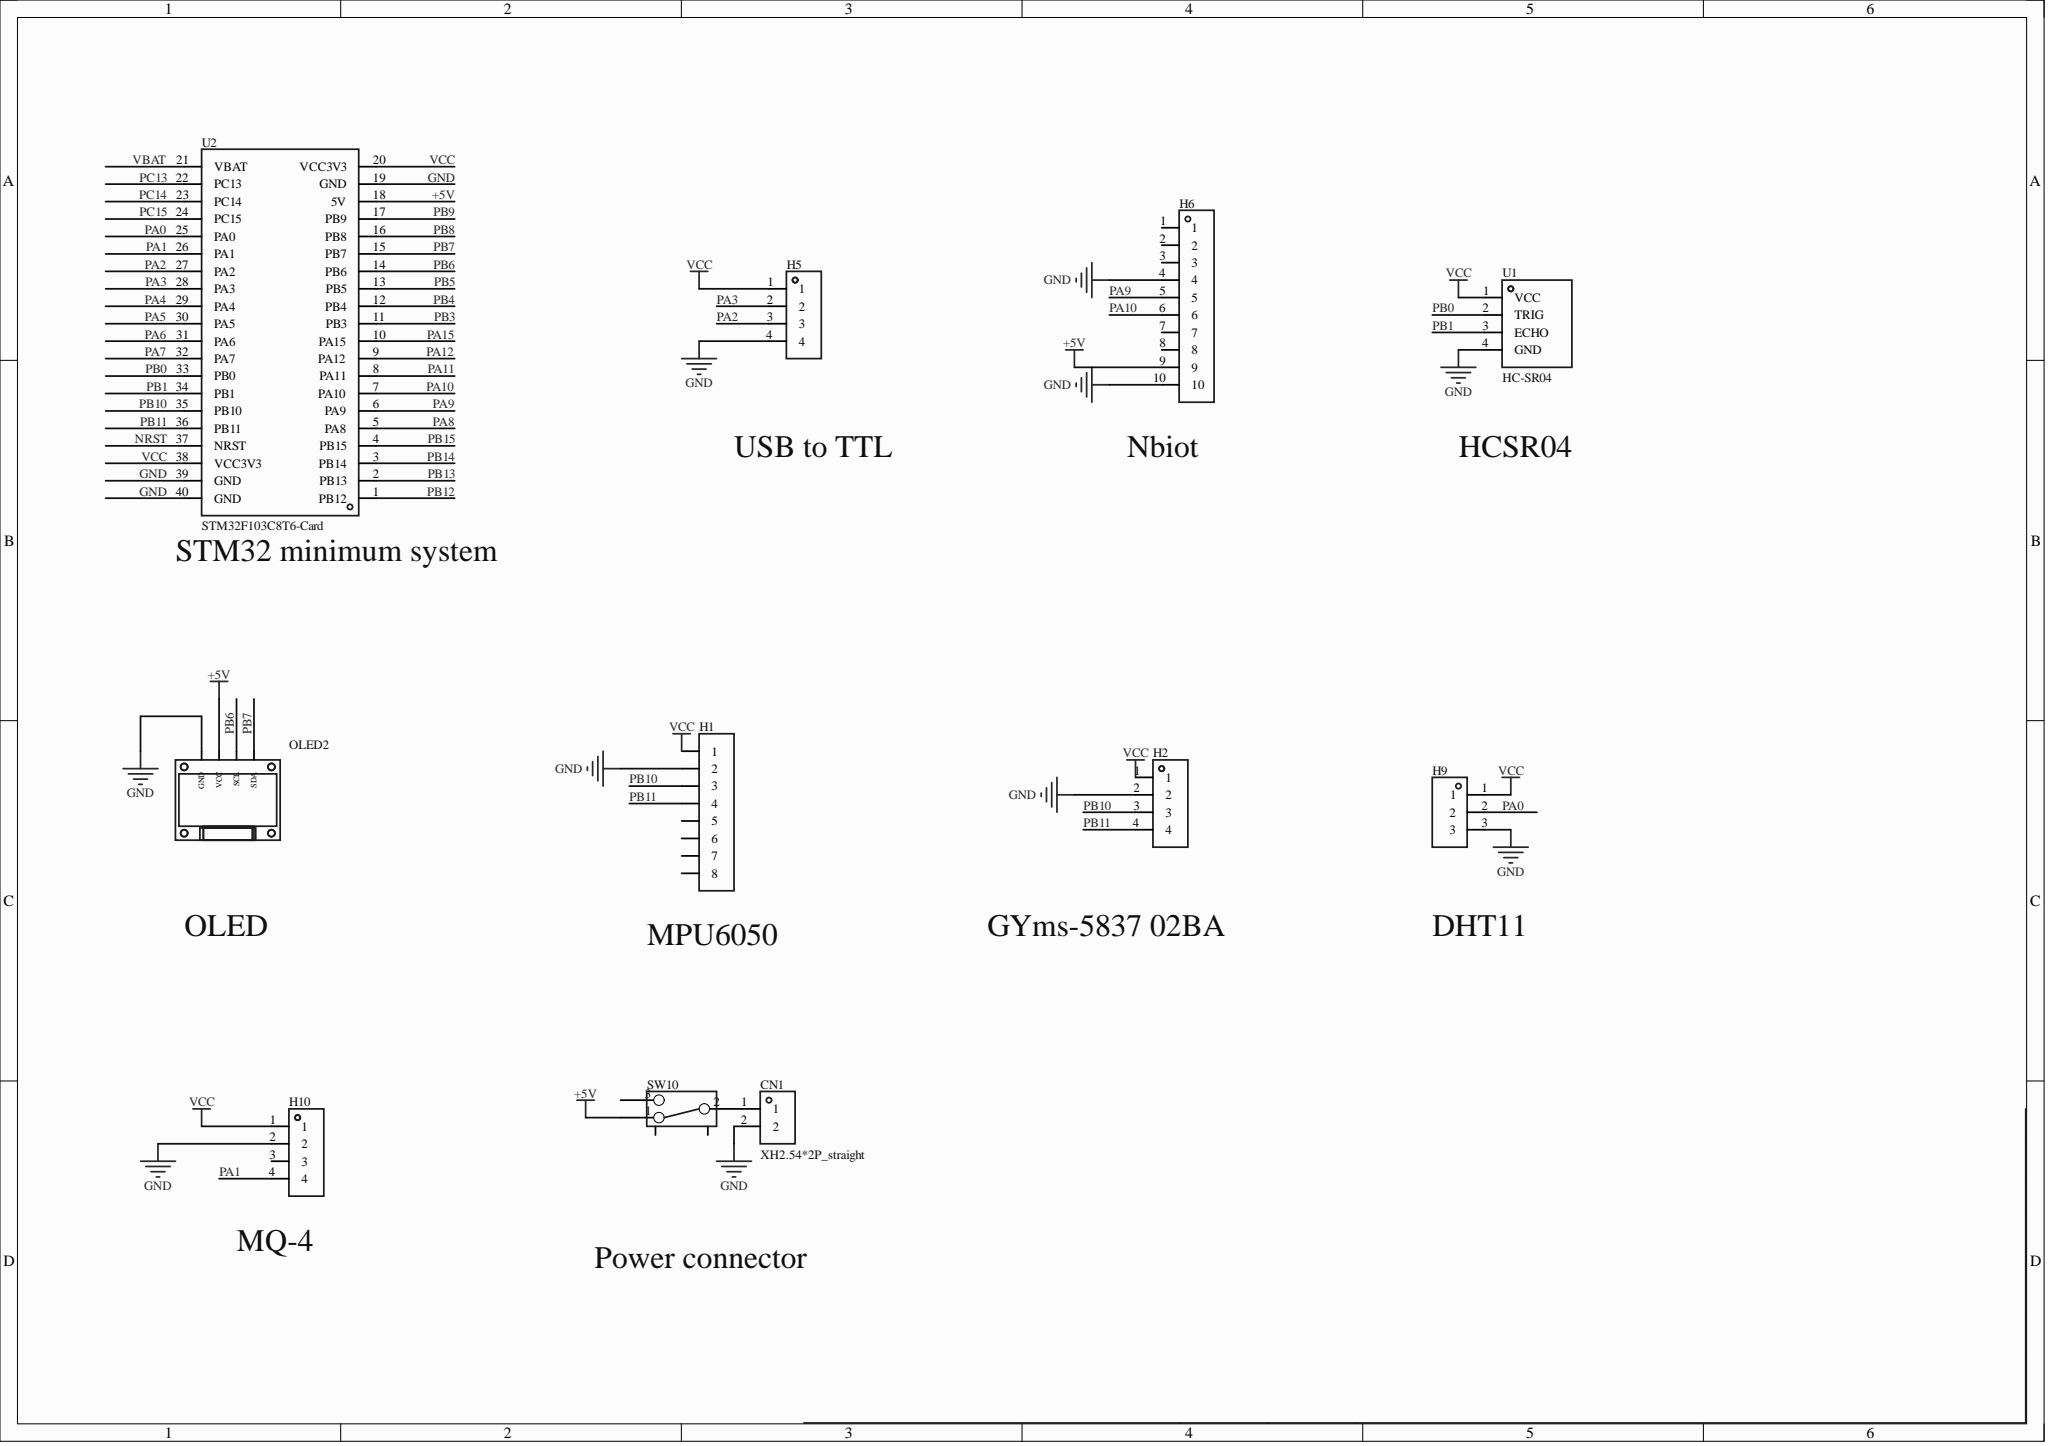Circuit board | Altium Designer | 11 parts | 16 nets
Bill of materials:
Comment,Description,Designator,Footprint,LibRef,Quantity
"XH2.54*2P_straight","","CN1","CONN-TH_2P-P2.50-XH2.54-2P","XH2.54*2P_直插","1"
"","","H1","HDR-TH_8P-P2.54-V-F-1","HDR-F_2.54_1x8P","1"
"","","H2, H5, H10","HDR-TH_4P-P2.54-V-F","HDR-F_2.54_1x4P","3"
"","","H6","HDR-TH_10P-P2.54-V-F","HDR-F_2.54_1x10P","1"
"","","H9","HDR-TH_3P-P2.54-V-F","HDR-F_2.54_1x3P","1"
"","","OLED2","0.96OLED_4P","0.96OLED模块_4P","1"
"","","SW10","拨动开关","拨动开关_正","1"
"HC-SR04","","U1","TH_HC-SR04V","HC-SR04","1"
"STM32F103C8T6-Card","","U2","CONN-TH_L53.3-W22.9_STM32F103C8T6-CARD","STM32F103C8T6-Card","1"
Netlist (Protel format):
[
CN1
CONN-TH_2P-P2.50-XH2.54-2P
XH2.54*2P_straight



]
[
H1
HDR-TH_8P-P2.54-V-F-1




]
[
H2
HDR-TH_4P-P2.54-V-F




]
[
H5
HDR-TH_4P-P2.54-V-F




]
[
H6
HDR-TH_10P-P2.54-V-F




]
[
H9
HDR-TH_3P-P2.54-V-F




]
[
H10
HDR-TH_4P-P2.54-V-F




]
[
OLED2
0.96OLED_4P




]
[
SW10
拨动开关




]
[
U1
TH_HC-SR04V
HC-SR04



]
[
U2
CONN-TH_L53.3-W22.9_STM32F103C8T6-CARD
STM32F103C8T6-Card



]
(
VCC
H1-1
H2-1
H5-1
H9-1
H10-1
U1-1
U2-20
U2-38
)
(
PB11
H1-4
H2-4
U2-36
)
(
PB10
H1-3
H2-3
U2-35
)
(
PB7
OLED2-4
U2-15
)
(
PB6
OLED2-3
U2-14
)
(
PB1
U1-3
U2-34
)
(
PB0
U1-2
U2-33
)
(
PA10
H6-6
U2-7
)
(
PA9
H6-5
U2-6
)
(
PA3
H5-2
U2-28
)
(
PA2
H5-3
U2-27
)
(
PA1
H10-4
U2-26
)
(
PA0
H9-2
U2-25
)
(
NetCN1_1
CN1-1
SW10-2
)
(
GND
CN1-2
H1-2
H2-2
H5-4
H6-4
H6-10
H9-3
H10-2
OLED2-1
U1-4
U2-19
U2-39
U2-40
)
(
+5V
H6-9
OLED2-2
SW10-1
U2-18
)